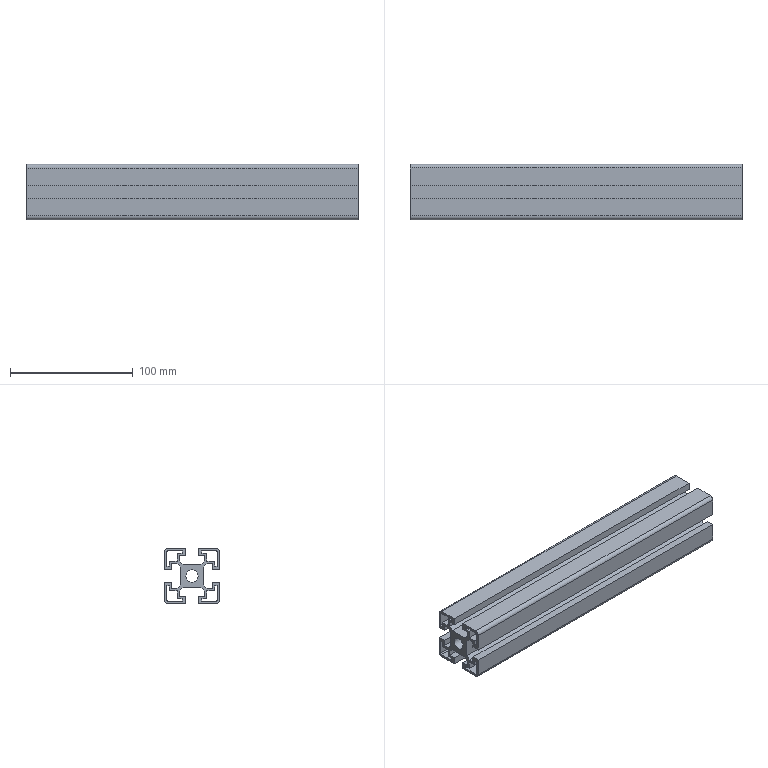Part | STEP file | 1_7 | 1 solid | 87 faces | box 270 x 45 x 45 mm | volume 220791 mm3 | plane 78 | cylinder 9 | commonest cylinder face diameters 2 x4 6 x4 10 x1